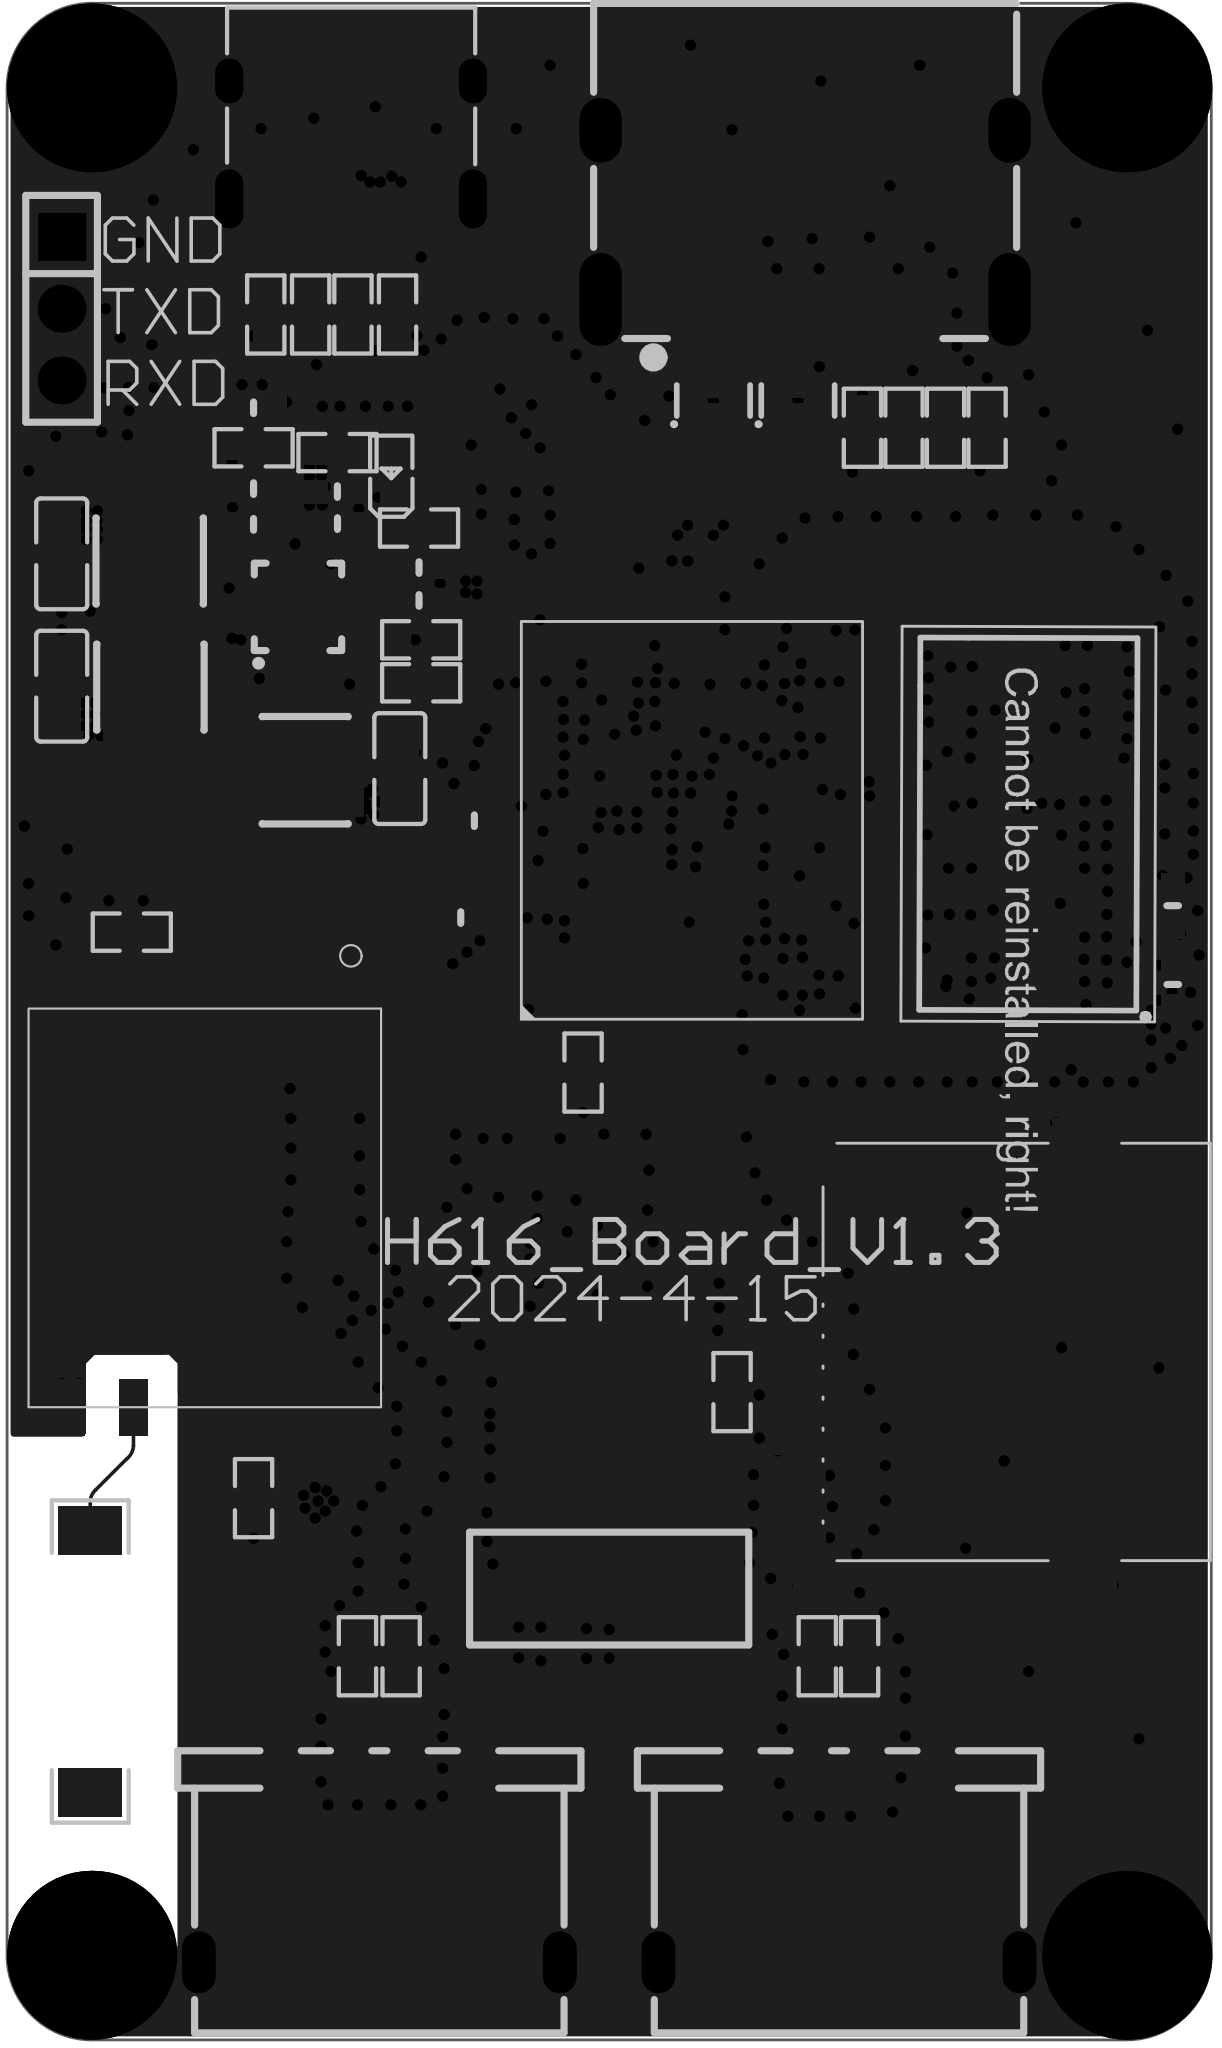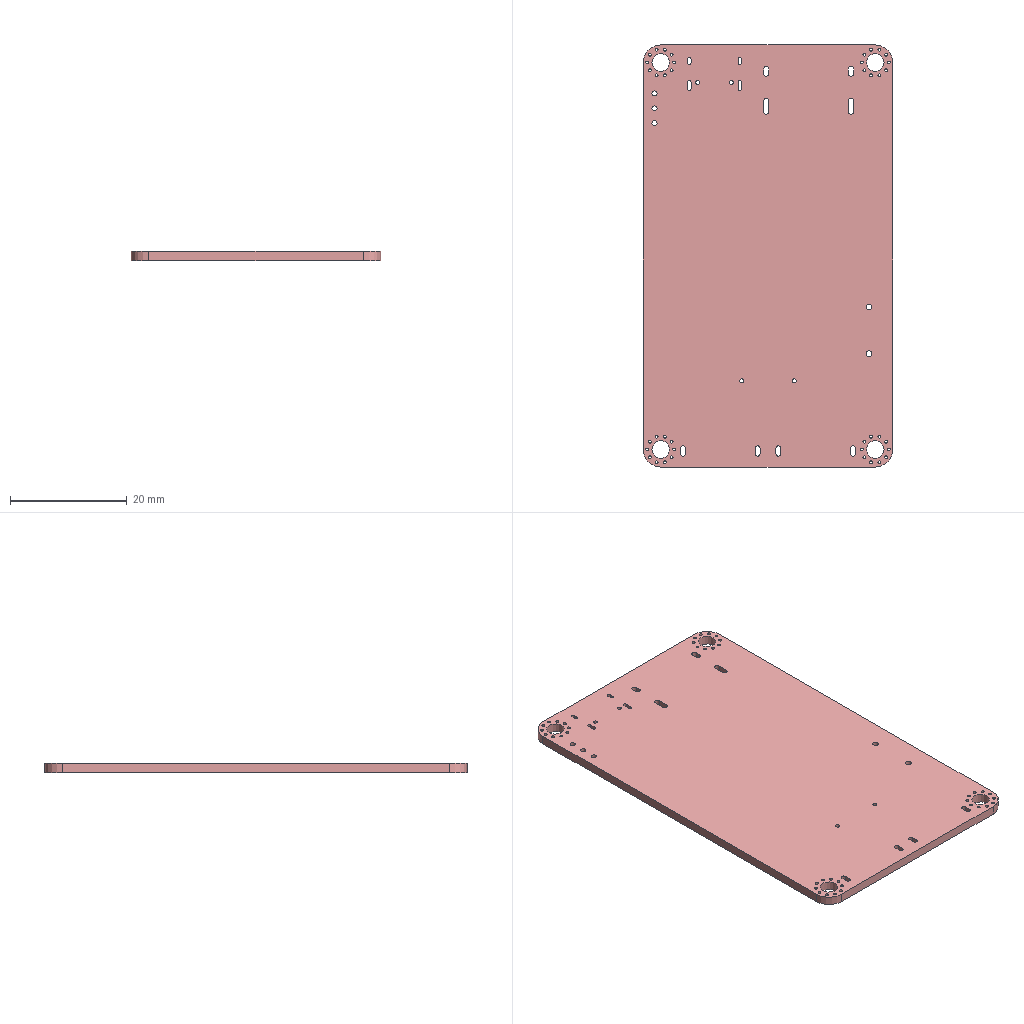Circuit board layout | Altium Designer | box 42.7 x 72.2 x 1.6 mm
Layer stack:
# Altium Designer layer stack of  (unit mm; dielectric type: 0 none, 1 core, 2 prepreg, 3 surface material)
index,name,kind,layer,copper_thickness_mm,dielectric_type,dielectric_thickness_mm,dielectric_material,dielectric_constant
0,Top Paste Mask Layer,other,,,,,,
1,Top Silkscreen Layer,other,,,,,,
2,Top Solder Mask Layer,dielectric,,,3,0,,0
3,Top Layer,copper,Top Layer,0.035,,,,
4,Dielectric1,dielectric,,,3,0.2104,7628 RC49% 8.6mil,0
5,GND,copper,GND,0.0152,,,,
6,Dielectric2,dielectric,,,3,1.065,1.1mm H/HOZ \u00BA\u00AC\u00CD\u00AD,0
7,PWR,copper,PWR,0.0152,,,,
8,Dielectric3,dielectric,,,3,0.2104,7628 RC49% 8.6mil,0
9,Bottom Layer,copper,Bottom Layer,0.035,,,,
10,Bottom Solder Mask Layer,dielectric,,,3,0,,0
11,Bottom Silkscreen Layer,other,,,,,,
12,Bottom Paste Mask Layer,other,,,,,,
# drill layer pairs: low layer,high layer
drill_pair,Top Layer,Bottom Layer
Part placement:
Designator,Comment,Layer,Footprint,Center-X(mm),Center-Y(mm),Rotation
D24,,TopLayer,SLP2510P8_L2.5-W1.0-P0.50-BL,103.429,135.636,0
D25,,TopLayer,SLP2510P8_L2.5-W1.0-P0.50-BL,106.426,135.636,0
U21,,TopLayer,BTB2X10,99.732,93.518,90
USB8,A/F board mount, type C, 10 (first two pins without curled edge), metal shell, LCP black glue=6.8,TopLayer,USB-A-SMD_C42496,91.582,84.018,0
USB9,A/F board mount, type C, 10 (first two pins without curled edge), metal shell, LCP black glue=6.8,TopLayer,USB-A-SMD_C42496,107.882,84.018,0
D26,,BottomLayer,SOD-323_L1.8-W1.3-LS2.5-NSK,110.541,132.385,180
D27,,BottomLayer,SOD-323_L1.8-W1.3-LS2.5-NSK,107.188,134.722,90
R117,10k,BottomLayer,R0603,111.658,134.671,90
U12,,TopLayer,WIFI模块,85.393,107.013,270
R118,100,TopLayer,R0603,111.658,134.671,90
R119,510,TopLayer,R0603,113.132,134.671,90
R120,27k,BottomLayer,R0603,108.712,134.671,90
R121,100,TopLayer,R0603,108.712,134.671,90
R122,10k,BottomLayer,R0603,110.185,134.671,90
R123,100,TopLayer,R0603,110.185,134.671,90
R124,100k,BottomLayer,R0603,113.132,134.671,90
USB10,HDMI 19PIN 043,TopLayer,HDMI-SMD_HDMI-19PIN-043,106.68,141.834,180
U5,,TopLayer,BGA284P65B1200_1400H125,102.667,120.752,90
U13,,TopLayer,M3_HOLE,81.382,80.518,0
U14,,TopLayer,M3_HOLE,118.082,80.518,0
U15,,TopLayer,M3_HOLE,118.082,146.718,0
U16,,TopLayer,M3_HOLE,81.382,146.718,0
R54,10K,TopLayer,R0603,90.098,133.789,180
R66,22R,TopLayer,R0603,90.646,138.686,90
R67,10K,TopLayer,R0603,89.146,138.686,90
R81,150K,BottomLayer,R0603,103.078,125.017,45
R6,,BottomLayer,R0402-NSK_2,104.255,124.153,0
R84,0,BottomLayer,R0603,101.351,128.98,0
R88,10K,TopLayer,R0603,92.355,91.118,270
R89,22R,TopLayer,R0603,90.806,91.118,270
R90,10K,TopLayer,R0603,108.611,91.118,270
R91,22R,TopLayer,R0603,107.111,91.118,270
C14,,TopLayer,C0603_NSK,87.122,131.242,0
C15,,TopLayer,C0603_NSK,87.122,132.512,0
C17,,BottomLayer,C0603_NSK,119.233,124.027,90
C18,,BottomLayer,C0603_NSK,118.166,115.01,225
C26,,BottomLayer,C0603_NSK,101.275,116.585,0
C27,,TopLayer,C0603_NSK,90.094,132.41,180
C22,,BottomLayer,C0603_NSK,101.028,121.683,180
C23,,BottomLayer,C0603_NSK,101.028,120.496,180
C24,,BottomLayer,C0603_NSK,100.538,118.541,90
C25,,BottomLayer,C0603_NSK,101.708,118.541,90
C100,,TopLayer,C0603_NSK,87.122,135.382,180
R49,,TopLayer,R0603,87.122,133.96,0
C12,,TopLayer,C0603_NSK,92.989,129.718,180
C5,,TopLayer,C0603_NSK,92.989,128.549,180
R3,,TopLayer,R0603,93.066,127.152,180
R2,,TopLayer,R0603,93.066,125.628,180
U9,AXP313A,TopLayer,WQFN-20_L3.0-W3.0-P0.40-BL-EP,88.697,128.321,0
R53,,TopLayer,R0603,92.989,131.115,180
C19,,TopLayer,C0603_NSK,119.715,114.933,270
LED2,,TopLayer,LED_0603,92.01,133.002,90
C116,,TopLayer,C0603_NSK,119.715,117.728,90
C118,,TopLayer,C0603_NSK,90.098,131.275,180
C120,,BottomLayer,C0603_NSK,118.217,117.474,90
C121,,BottomLayer,C0603_NSK,106.25,120.201,180
C122,,BottomLayer,C0603_NSK,103.644,118.827,0
C123,,BottomLayer,C0603_NSK,119.233,126.592,270
R26,6.04k,BottomLayer,R0603,96.672,127.152,90
C124,,BottomLayer,C0603_NSK,103.51,121.791,315
C125,,BottomLayer,C0603_NSK,116.644,112.802,45
C126,,BottomLayer,C0603_NSK,103.644,119.995,0
L4,1uH,TopLayer,IND-SMD_L3.0-W3.0,83.439,129.946,270
L5,1uH,TopLayer,IND-SMD_L3.0-W3.0,83.464,125.476,90
L6,1uH,TopLayer,IND-SMD_L3.0-W3.0,88.951,122.53,180
C136,47uF,TopLayer,C0805,80.319,125.509,90
C137,47uF,TopLayer,C0805,92.308,122.588,270
C138,47uF,TopLayer,C0805,80.319,130.2,270
C139,47uF,BottomLayer,C0805,87.609,128.354,180
C140,47uF,BottomLayer,C0805,83.85,128.354,0
C141,47uF,BottomLayer,C0805,87.609,126.195,180
C143,,BottomLayer,C0603_NSK,98.167,119.276,0
C144,,BottomLayer,C0603_NSK,101.588,123.594,135
C94,,TopLayer,C0603_NSK,94.469,117.309,180
C99,,TopLayer,C0603_NSK,94.952,120.738,0
X2,24M,TopLayer,OSC-SMD_4P-L2.0-W1.6-BL,94.897,118.983,90
USB3,,TopLayer,USB-C-SMD_TYPEC-304-BCP16-1,90.582,144.418,180
R43,,TopLayer,R0603,87.555,138.686,270
R70,,TopLayer,R0603,92.228,138.686,90
C105,2.2UF,BottomLayer,C0603,97.922,127.202,270
C106,1UF,BottomLayer,C0603,96.678,123.951,0
C108,220NF,BottomLayer,C0603,99.784,123.543,90
C130,2.2uF,BottomLayer,C0603,102.266,127.126,270
C131,2.2uF,BottomLayer,C0603,99.924,126.594,270
C132,100nF,BottomLayer,C0603,98.159,120.673,180
R52,,TopLayer,R0603,98.806,111.811,270
H4,,TopLayer,hdr-th_3p-p2.54-v-m,80.315,138.887,270
CARD1,TF-015,TopLayer,TF-SMD_TF-015,111.506,101.803,90
R18,10Ω,TopLayer,R0603,104.089,100.482,270
C133,,BottomLayer,C0603_NSK,104.343,99.619,90
R87,0Ω,TopLayer,R0603,87.122,96.723,90
U6,,TopLayer,FBGA96,114.594,120.621,179.8
R10,240,BottomLayer,R0402,113.696,122.934,180
R11,240,BottomLayer,R0402,110.216,122.68,0
R12,100,BottomLayer,R0402,114.243,121.77,45
R55,2K,BottomLayer,R0402,118.693,119.175,180
R56,2K,BottomLayer,R0402,118.693,119.937,0
C129,100nF,BottomLayer,C0402,118.693,121.487,180
C128,100nF,BottomLayer,C0402,118.693,120.699,180
C127,100nF,BottomLayer,C0402,118.693,122.292,180
U22,AN9520,TopLayer,ANT-SMD_L9.5-W2.1,81.331,90.932,270
R86,10Ω,TopLayer,R0603,82.804,116.789,0
Pad and via stacks:
# Altium Designer via and pad stacks of  (unit mm). Each distinct definition once, with the count of objects using it.
# via: kind,start_layer,end_layer,hole_mm,diameter_mm,mode(0 simple;1 top-mid-bottom;2 full stack),diameter_per_layer,count,example_net
# pad: kind,layer,hole_mm,hole_type(0 round;1 square;2 slot),plating,top_size,top_shape(1 round;2 rect;3 octagon;9 rounded rect),mid_size,bottom_size,mode,footprint,size_per_layer,count,example
pad,Top Layer,0,0,plated,0.2007x0.6807,2,0.2007x0.6807,0.2007x0.6807,0,SLP2510P8_L2.5-W1.0-P0.50-BL,,16,D24.10
pad,Top Layer,0,0,plated,0.3988x0.6807,2,0.3988x0.6807,0.3988x0.6807,0,SLP2510P8_L2.5-W1.0-P0.50-BL,,4,D24.8
pad,Top Layer,0,0,plated,0.3x2,2,0.3x2,0.3x2,0,BTB2X10,,20,U21.1
pad,Top Layer,0,0,plated,1x2.6,2,1x2.6,1x2.6,0,USB-A-SMD_C42496,,8,USB8.1
pad,Top Layer,0,0,plated,2x1,2,2x1,2x1,0,WIFI\u00C4\u00A3\u00BF\u00E9,,13,U12.1
pad,Top Layer,0,0,plated,0.8065x0.864,2,0.8065x0.864,0.8065x0.864,0,R0603,,42,R118.2
pad,Top Layer,0,0,plated,0.3x2.6,2,0.3x2.6,0.3x2.6,0,HDMI-SMD_HDMI-19PIN-043,,19,USB10.19
pad,Top Layer,0,0,plated,0.254x0.254,1,0.254x0.254,0.254x0.254,0,BGA284P65B1200_1400H125,,284,U5.V21
pad,Top Layer,0,0,plated,0.85x0.85,2,0.85x0.85,0.85x0.85,0,C0603 NSK,,22,C14.2
pad,Top Layer,0,0,plated,0.2007x0.8001,2,0.2007x0.8001,0.2007x0.8001,0,WQFN-20_L3.0-W3.0-P0.40-BL-EP,,20,U9.1
pad,Top Layer,0,0,plated,1.699x1.699,2,1.699x1.699,1.699x1.699,0,WQFN-20_L3.0-W3.0-P0.40-BL-EP,,1,U9.21
pad,Top Layer,0,0,plated,0.8001x0.8001,2,0.8001x0.8001,0.8001x0.8001,0,LED_0603,,2,LED2.1
pad,Top Layer,0,0,plated,1.5x3.32,2,1.5x3.32,1.5x3.32,0,IND-SMD_L3.0-W3.0,,6,L4.1
pad,Top Layer,0,0,plated,1.41x1.35,2,1.41x1.35,1.41x1.35,0,C0805,,6,C136.2
pad,Top Layer,0,0,plated,0.762x0.508,2,0.762x0.508,0.762x0.508,0,OSC-SMD_4P-L2.0-W1.6-BL,,4,X2.1
pad,Top Layer,0,0,plated,0.5512x1.45,2,0.5512x1.45,0.5512x1.45,0,USB-C-SMD_TYPEC-304-BCP16-1,,4,USB3.A1B12
pad,Top Layer,0,0,plated,0.2997x1.45,2,0.2997x1.45,0.2997x1.45,0,USB-C-SMD_TYPEC-304-BCP16-1,,8,USB3.B8
pad,Top Layer,0,0,plated,0.701x1.999,2,0.701x1.999,0.701x1.999,0,TF-SMD_TF-015,,9,CARD1.1
pad,Top Layer,0,0,plated,1.199x1.397,2,1.199x1.397,1.199x1.397,0,TF-SMD_TF-015,,1,CARD1.10
pad,Top Layer,0,0,plated,1.778x1.397,2,1.778x1.397,1.778x1.397,0,TF-SMD_TF-015,,1,CARD1.13
pad,Top Layer,0,0,plated,1.27x2.286,2,1.27x2.286,1.27x2.286,0,TF-SMD_TF-015,,2,CARD1.12
pad,Top Layer,0,0,plated,0.3556x0.3556,1,0.3556x0.3556,0.3556x0.3556,0,FBGA96,,96,U6.A1
pad,Top Layer,0,0,plated,1.71x2.268,2,1.71x2.268,1.71x2.268,0,ANT-SMD_L9.5-W2.1,,2,U22.2
pad,Multi-Layer,0.8,2,plated,2.2x1.2,1,2.2x1.2,2.2x1.2,0,USB-A-SMD_C42496,,4,USB8.5
pad,Multi-Layer,0.9,2,plated,1.5x3.3,1,1.5x3.3,1.5x3.3,0,HDMI-SMD_HDMI-19PIN-043,,2,USB10.20
pad,Multi-Layer,0.9,2,plated,1.5x2.3,1,1.5x2.3,1.5x2.3,0,HDMI-SMD_HDMI-19PIN-043,,2,USB10.20
pad,Multi-Layer,3,0,plated,6x6,1,6x6,6x6,0,M3_HOLE,,4,U13.1
pad,Multi-Layer,0.5,0,plated,1x1,1,1x1,1x1,0,M3_HOLE,,40,U13.1
pad,Multi-Layer,0.5994,2,plated,1.001x2.101,1,1.001x2.101,1.001x2.101,0,USB-C-SMD_TYPEC-304-BCP16-1,,2,USB3.12
pad,Multi-Layer,0.5994,2,plated,1.001x1.6,1,1.001x1.6,1.001x1.6,0,USB-C-SMD_TYPEC-304-BCP16-1,,2,USB3.14
pad,Multi-Layer,0.889,0,plated,1.7x1.7,2,1.7x1.7,1.7x1.7,0,hdr-th_3p-p2.54-v-m,,1,H4.1
pad,Multi-Layer,0.889,0,plated,1.7x1.7,1,1.7x1.7,1.7x1.7,0,hdr-th_3p-p2.54-v-m,,2,H4.2
pad,Bottom Layer,0,0,plated,0.8458x0.4547,2,0.8458x0.4547,0.8458x0.4547,0,SOD-323_L1.8-W1.3-LS2.5-NSK,,4,D26.2
pad,Bottom Layer,0,0,plated,0.8065x0.864,2,0.8065x0.864,0.8065x0.864,0,R0603,,14,R117.2
pad,Bottom Layer,0,0,plated,0.5x0.5588,2,0.5x0.5588,0.5x0.5588,0,R0402-NSK_2,,2,R6.2
pad,Bottom Layer,0,0,plated,0.85x0.85,2,0.85x0.85,0.85x0.85,0,C0603 NSK,,34,C17.2
pad,Bottom Layer,0,0,plated,1.41x1.35,2,1.41x1.35,1.41x1.35,0,C0805,,6,C139.2
pad,Bottom Layer,0,0,plated,0.8x0.9,2,0.8x0.9,0.8x0.9,0,C0603,,12,C105.2
pad,Bottom Layer,0,0,plated,0.5657x0.54,2,0.5657x0.54,0.5657x0.54,0,R0402,,10,R10.2
pad,Bottom Layer,0,0,plated,0.7901x0.54,2,0.7901x0.54,0.7901x0.54,0,C0402,,6,C129.2
via,Top Layer,Bottom Layer,0.2997,0.3988,0,,611,SA1
Copper pours:
name,layer,net,type(0 solid;1 hatched;2 none)
Top Layer-VDD_GPU,Top Layer,VDD_GPU,0
Top Layer-1V8,Top Layer,1V8,0
Top Layer-3V3,Top Layer,3V3,0
Top Layer-GND,Top Layer,GND,0
Top Layer-VDD_CPU,Top Layer,VDD_CPU,0
Top Layer-1V8 1,Top Layer,1V8,0
Top Layer-$2N1522,Top Layer,$2N1522,0
Top Layer-VCC_DRAM,Top Layer,VCC_DRAM,0
Top Layer-VDD_CPU 1,Top Layer,VDD_CPU,0
Top Layer-PS,Top Layer,PS,0
Top Layer-PS 1,Top Layer,PS,0
Top Layer-$2N1523,Top Layer,$2N1523,0
Top Layer-VDD_GPU 1,Top Layer,VDD_GPU,0
Top Layer-$2N1524,Top Layer,$2N1524,0
Top Layer-PS 2,Top Layer,PS,0
Top Layer-1V8 2,Top Layer,1V8,0
Top Layer-3V3 1,Top Layer,3V3,0
Top Layer-PS 3,Top Layer,PS,0
Top Layer-GND 1,Top Layer,GND,0
Top Layer-3V3 2,Top Layer,3V3,0
Top Layer-PS 4,Top Layer,PS,0
Top Layer-GND 2,Top Layer,GND,0
Bottom Layer-1V8,Bottom Layer,1V8,0
Bottom Layer-3V3,Bottom Layer,3V3,0
Bottom Layer-PS,Bottom Layer,PS,0
Bottom Layer-PS 1,Bottom Layer,PS,0
Bottom Layer-GND,Bottom Layer,GND,0
PWR-VCC_DRAM,PWR,VCC_DRAM,0
PWR-VDD_CPU,PWR,VDD_CPU,0
PWR-VDD_GPU,PWR,VDD_GPU,0
PWR-1V8,PWR,1V8,0
PWR-VCC_DRAM 1,PWR,VCC_DRAM,0
PWR-3V3,PWR,3V3,0
Design rules, without the lines most boards share:
# Altium Designer design rules of  (exported by Altium Designer, unit mm)
# columns: name | kind | enabled | priority | scope1 | scope2 | descriptor | typed fields (field=value)
safeClearance | 0 | disabled | 1 | All | All | Clearance Constraint (Gap=4mil) (Disabled)(All),(All) | gap=0.1016
safeClearance_1 | 63 | disabled | 1 | All | All | Board Clearance Constraint (Gap=0mil) (Disabled)(All) |
copperThicknessInner0.5oz | 0 | disabled | 2 | All | All | Clearance Constraint (Gap=4mil) (Disabled)(All),(All) | gap=0.1016
copperThicknessInner0.5oz_1 | 63 | disabled | 2 | All | All | Board Clearance Constraint (Gap=0mil) (Disabled)(All) |
Plane_innerPlane | 0 | disabled | 3 | All | All | Clearance Constraint (Gap=4mil) (Disabled)(All),(All) | gap=0.1016
Plane_innerPlane_1 | 63 | disabled | 3 | All | All | Board Clearance Constraint (Gap=0mil) (Disabled)(All) |
Copper_copperRegion | 0 | disabled | 4 | All | All | Clearance Constraint (Gap=4mil) (Disabled)(All),(All) | gap=0.1016
Copper_copperRegion_1 | 63 | disabled | 4 | All | All | Board Clearance Constraint (Gap=0mil) (Disabled)(All) |
Clearance | 0 | disabled | 5 | All | All | Clearance Constraint (Gap=4mil) (Disabled)(All),(All) | gap=0.1016
BoardOutlineClearance | 63 | disabled | 5 | All | All | Board Clearance Constraint (Gap=0mil) (Disabled)(All) |
Clearance_1 | 0 | disabled | 6 | All | All | Clearance Constraint (Gap=4mil) (Disabled)(All),(All) | gap=0.1016
BoardOutlineClearance_1 | 63 | disabled | 6 | All | All | Board Clearance Constraint (Gap=0mil) (Disabled)(All) |
copperThickness1oz | 0 | enabled | 7 | All | All | Clearance Constraint (Gap=4mil) (All),(All) | gap=0.1016
copperThickness1oz_1 | 63 | enabled | 7 | All | All | Board Clearance Constraint (Gap=0mil) (All) |
otherClearance | 52 | enabled | 1 | All | All | Hole To Hole Clearance (Gap=11.8mil) (All),(All) | gap=0.2997
trackWidth | 2 | disabled | 1 | All | All | Width Constraint (Min=4mil) (Max=100mil) (Preferred=5mil) (Disabled)(All) |
copperThickness2oz | 2 | disabled | 2 | All | All | Width Constraint (Min=4mil) (Max=100mil) (Preferred=10mil) (Disabled)(All) |
copperThickness0.5oz | 2 | disabled | 3 | All | All | Width Constraint (Min=4mil) (Max=100mil) (Preferred=10mil) (Disabled)(All) |
copperThickness1oz_2 | 2 | enabled | 4 | All | All | Width Constraint (Min=4mil) (Max=100mil) (Preferred=5mil) (All) |
nei | 51 | disabled | 1 | All | All | Differential Pairs Uncoupled Length using the Gap Constraints (Min=7mil) (Max=7mil) (Prefered=7mil)  and Width Constraints (Min=4mil) (Max=10mil) (Prefered=4mil) (Disabled)(All) |
wai | 51 | enabled | 2 | All | All | Differential Pairs Uncoupled Length using the Gap Constraints (Min=5mil) (Max=5mil) (Prefered=5mil)  and Width Constraints (Min=4mil) (Max=100mil) (Prefered=4mil) (All) |
viaSize | 11 | enabled | 1 | All | All | Routing Via (MinHoleWidth=11.8mil) (MaxHoleWidth=236.2mil) (PreferredHoleWidth=11.8mil) (MinWidth=15.7mil) (MaxWidth=393.7mil) (PreferedWidth=15.7mil) (All) | via_min_hole=0.2997 via_max_hole=6 via_preferred_diameter=0.3988 via_preferred_hole=0.2997
innerPlane | 6 | enabled | 1 | All | All | Power Plane Connect Rule(Direct Connect )(Expansion=20mil) (Conductor Width=10mil) (Air Gap=10mil) (Entries=4) (All) | relief_conductor_width=0.254 relief_entries=4 relief_expansion=0.508
copperRegion | 20 | disabled | 1 | All | All | Polygon Connect Rule(Relief Connect )(Conductor Width=10mil) (Relief Angle=90 Angle) (Entries=4) (Air Gap Width=10mil) (Disabled)(All),(All) | connect_style(0=relief,1=direct,2=none)=0 relief_conductor_width=0.254 relief_entries=4
PolygonConnect | 20 | disabled | 2 | All | All | Polygon Connect Rule(Direct Connect )(Conductor Width=10mil) (Relief Angle=90 Angle) (Entries=4) (Air Gap Width=10mil) (Disabled)(All),(All) | connect_style(0=relief,1=direct,2=none)=1 relief_conductor_width=0.254 relief_entries=4
PolygonConnect_1 | 20 | enabled | 3 | All | All | Polygon Connect Rule(Direct Connect )(Conductor Width=10mil) (Relief Angle=90 Angle) (Entries=4) (Air Gap Width=10mil) (All),(All) | connect_style(0=relief,1=direct,2=none)=1 relief_conductor_width=0.254 relief_entries=4
solderMaskExpansion | 13 | enabled | 2 | All | All | Solder Mask Expansion (Expansion =4mil) (All) | expansion=0.1016